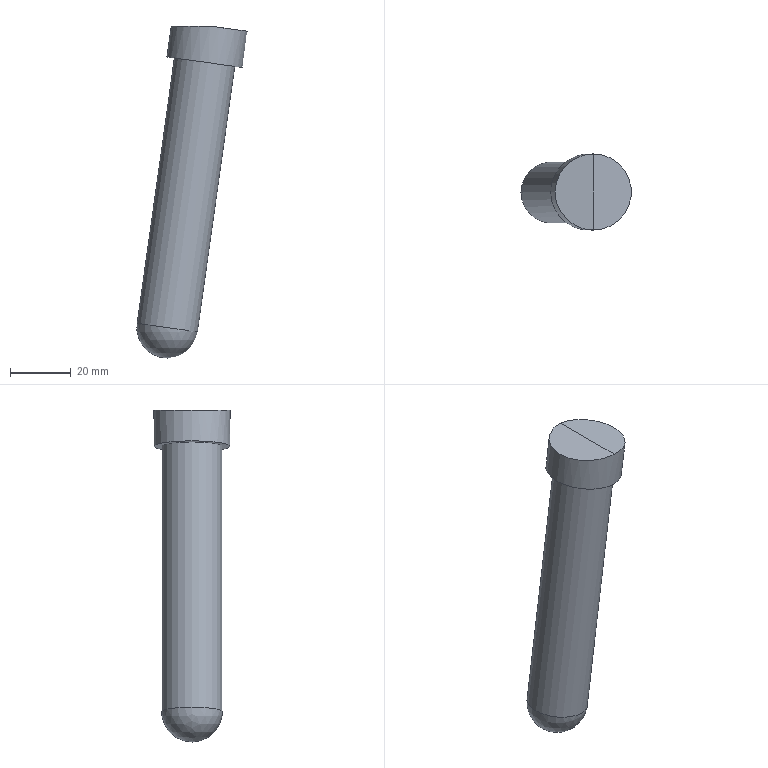Part | STEP file | P011002S003-011 | 1 solid | 6 faces | box 36.296 x 25 x 109.027 mm | volume 35448 mm3 | plane 3 | cylinder 2 | sphere 1 | commonest cylinder face diameters 20 x1 25 x1
STEP:
#1=CARTESIAN_POINT('',(0.,0.,0.));
#2=DIRECTION('',(0.,0.,1.));
#3=DIRECTION('',(1.,0.,0.));
#4=AXIS2_PLACEMENT_3D('',#1,#2,#3);
#5=CARTESIAN_POINT('',(-193.,-46.5,75.));
#6=VERTEX_POINT('',#5);
#7=CARTESIAN_POINT('',(-193.,-71.5,75.));
#8=VERTEX_POINT('',#7);
#9=CARTESIAN_POINT('',(-193.,-59.,75.));
#10=DIRECTION('',(0.,-1.,0.));
#11=VECTOR('',#10,1.);
#12=LINE('',#9,#11);
#13=CARTESIAN_POINT('',(-193.,-59.,75.));
#14=DIRECTION('',(-0.1392,0.,-0.9903));
#15=DIRECTION('',(0.9903,0.,-0.1392));
#16=AXIS2_PLACEMENT_3D('',#13,#14,#15);
#17=PLANE('',#16);
#18=CARTESIAN_POINT('',(0.,0.));
#19=DIRECTION('',(0.,1.));
#20=VECTOR('',#19,1.);
#21=LINE('',#18,#20);
#22=(GEOMETRIC_REPRESENTATION_CONTEXT(2)PARAMETRIC_REPRESENTATION_CONTEXT()REPRESENTATION_CONTEXT('',''));
#23=DEFINITIONAL_REPRESENTATION('',(#21),#22);
#24=PCURVE('',#17,#23);
#25=CARTESIAN_POINT('',(-250.,-9.,75.));
#26=DIRECTION('',(0.,0.,1.));
#27=DIRECTION('',(-1.,0.,0.));
#28=AXIS2_PLACEMENT_3D('',#25,#26,#27);
#29=PLANE('',#28);
#30=CARTESIAN_POINT('',(-57.,50.));
#31=DIRECTION('',(0.,1.));
#32=VECTOR('',#31,1.);
#33=LINE('',#30,#32);
#34=(GEOMETRIC_REPRESENTATION_CONTEXT(2)PARAMETRIC_REPRESENTATION_CONTEXT()REPRESENTATION_CONTEXT('',''));
#35=DEFINITIONAL_REPRESENTATION('',(#33),#34);
#36=PCURVE('',#29,#35);
#37=SURFACE_CURVE('',#12,(#24,#36),.PCURVE_S1.);
#38=EDGE_CURVE('',#6,#8,#37,.T.);
#39=ORIENTED_EDGE('',*,*,#38,.T.);
#40=CARTESIAN_POINT('',(-193.,-59.,75.));
#41=DIRECTION('',(0.1392,0.,0.9903));
#42=DIRECTION('',(0.9903,0.,-0.1392));
#43=AXIS2_PLACEMENT_3D('',#40,#41,#42);
#44=CIRCLE('',#43,12.5);
#45=CARTESIAN_POINT('',(12.5,0.));
#46=CARTESIAN_POINT('',(12.5,-21.651));
#47=CARTESIAN_POINT('',(-6.25,-10.825));
#48=CARTESIAN_POINT('',(-25.,0.));
#49=CARTESIAN_POINT('',(-6.25,10.825));
#50=CARTESIAN_POINT('',(12.5,21.651));
#51=CARTESIAN_POINT('',(12.5,0.));
#52=(BOUNDED_CURVE()B_SPLINE_CURVE(2,(#45,#46,#47,#48,#49,#50,#51),.UNSPECIFIED.,.T.,.F.)B_SPLINE_CURVE_WITH_KNOTS((1,2,2,2,2,1),(-2.094,0.,2.094,4.189,6.283,8.378),.UNSPECIFIED.)CURVE()GEOMETRIC_REPRESENTATION_ITEM()RATIONAL_B_SPLINE_CURVE((1.,0.5,1.,0.5,1.,0.5,1.))REPRESENTATION_ITEM(''));
#53=(GEOMETRIC_REPRESENTATION_CONTEXT(2)PARAMETRIC_REPRESENTATION_CONTEXT()REPRESENTATION_CONTEXT('',''));
#54=DEFINITIONAL_REPRESENTATION('',(#52),#53);
#55=PCURVE('',#17,#54);
#56=CARTESIAN_POINT('',(-222.706,-59.,-136.373));
#57=DIRECTION('',(0.1392,0.,0.9903));
#58=DIRECTION('',(-0.9903,0.,0.1392));
#59=AXIS2_PLACEMENT_3D('',#56,#57,#58);
#60=CYLINDRICAL_SURFACE('',#59,12.5);
#61=CARTESIAN_POINT('',(-3.142,213.45));
#62=DIRECTION('',(1.,0.));
#63=VECTOR('',#62,1.);
#64=LINE('',#61,#63);
#65=(GEOMETRIC_REPRESENTATION_CONTEXT(2)PARAMETRIC_REPRESENTATION_CONTEXT()REPRESENTATION_CONTEXT('',''));
#66=DEFINITIONAL_REPRESENTATION('',(#64),#65);
#67=PCURVE('',#60,#66);
#68=SURFACE_CURVE('',#44,(#55,#67),.PCURVE_S1.);
#69=EDGE_CURVE('',#8,#6,#68,.T.);
#70=ORIENTED_EDGE('',*,*,#69,.T.);
#71=EDGE_LOOP('',(#39,#70));
#72=FACE_BOUND('',#71,.T.);
#73=ADVANCED_FACE('',(#72),#17,.F.);
#74=CARTESIAN_POINT('',(-207.048,-59.,64.856));
#75=VERTEX_POINT('',#74);
#76=CARTESIAN_POINT('',(-194.67,-59.,63.117));
#77=DIRECTION('',(-0.1392,0.,-0.9903));
#78=DIRECTION('',(-0.9903,0.,0.1392));
#79=AXIS2_PLACEMENT_3D('',#76,#77,#78);
#80=CIRCLE('',#79,12.5);
#81=CARTESIAN_POINT('',(6.283,201.45));
#82=DIRECTION('',(-1.,0.));
#83=VECTOR('',#82,1.);
#84=LINE('',#81,#83);
#85=(GEOMETRIC_REPRESENTATION_CONTEXT(2)PARAMETRIC_REPRESENTATION_CONTEXT()REPRESENTATION_CONTEXT('',''));
#86=DEFINITIONAL_REPRESENTATION('',(#84),#85);
#87=PCURVE('',#60,#86);
#88=CARTESIAN_POINT('',(-194.67,-109.,63.117));
#89=DIRECTION('',(0.1392,0.,0.9903));
#90=DIRECTION('',(-0.9903,0.,0.1392));
#91=AXIS2_PLACEMENT_3D('',#88,#89,#90);
#92=PLANE('',#91);
#93=CARTESIAN_POINT('',(12.5,-50.));
#94=CARTESIAN_POINT('',(12.5,-71.651));
#95=CARTESIAN_POINT('',(-6.25,-60.825));
#96=CARTESIAN_POINT('',(-25.,-50.));
#97=CARTESIAN_POINT('',(-6.25,-39.175));
#98=CARTESIAN_POINT('',(12.5,-28.349));
#99=CARTESIAN_POINT('',(12.5,-50.));
#100=(BOUNDED_CURVE()B_SPLINE_CURVE(2,(#93,#94,#95,#96,#97,#98,#99),.UNSPECIFIED.,.T.,.F.)B_SPLINE_CURVE_WITH_KNOTS((1,2,2,2,2,1),(-2.094,0.,2.094,4.189,6.283,8.378),.UNSPECIFIED.)CURVE()GEOMETRIC_REPRESENTATION_ITEM()RATIONAL_B_SPLINE_CURVE((1.,0.5,1.,0.5,1.,0.5,1.))REPRESENTATION_ITEM(''));
#101=(GEOMETRIC_REPRESENTATION_CONTEXT(2)PARAMETRIC_REPRESENTATION_CONTEXT()REPRESENTATION_CONTEXT('',''));
#102=DEFINITIONAL_REPRESENTATION('',(#100),#101);
#103=PCURVE('',#92,#102);
#104=SURFACE_CURVE('',#80,(#87,#103),.PCURVE_S1.);
#105=EDGE_CURVE('',#75,#75,#104,.T.);
#106=ORIENTED_EDGE('',*,*,#105,.F.);
#107=CARTESIAN_POINT('',(-205.623,-59.,75.));
#108=VERTEX_POINT('',#107);
#109=CARTESIAN_POINT('',(-207.048,-59.,64.856));
#110=CARTESIAN_POINT('',(-205.623,-59.,75.));
#111=B_SPLINE_CURVE_WITH_KNOTS('',1,(#109,#110),.UNSPECIFIED.,.F.,.F.,(2,2),(201.45,211.693),.PIECEWISE_BEZIER_KNOTS.);
#112=CARTESIAN_POINT('',(6.283,0.));
#113=DIRECTION('',(0.,1.));
#114=VECTOR('',#113,1.);
#115=LINE('',#112,#114);
#116=(GEOMETRIC_REPRESENTATION_CONTEXT(2)PARAMETRIC_REPRESENTATION_CONTEXT()REPRESENTATION_CONTEXT('',''));
#117=DEFINITIONAL_REPRESENTATION('',(#115),#116);
#118=PCURVE('',#60,#117);
#119=CARTESIAN_POINT('',(0.,0.));
#120=DIRECTION('',(0.,1.));
#121=VECTOR('',#120,1.);
#122=LINE('',#119,#121);
#123=(GEOMETRIC_REPRESENTATION_CONTEXT(2)PARAMETRIC_REPRESENTATION_CONTEXT()REPRESENTATION_CONTEXT('',''));
#124=DEFINITIONAL_REPRESENTATION('',(#122),#123);
#125=PCURVE('',#60,#124);
#126=SEAM_CURVE('',#111,(#118,#125),.PCURVE_S1.);
#127=EDGE_CURVE('',#75,#108,#126,.T.);
#128=ORIENTED_EDGE('',*,*,#127,.T.);
#129=CARTESIAN_POINT('',(-193.,-59.,75.));
#130=DIRECTION('',(0.,0.,-1.));
#131=DIRECTION('',(1.,0.,0.));
#132=AXIS2_PLACEMENT_3D('',#129,#130,#131);
#133=ELLIPSE('',#132,12.623,12.5);
#134=CARTESIAN_POINT('',(7.854,213.45));
#135=CARTESIAN_POINT('',(7.806,213.366));
#136=CARTESIAN_POINT('',(7.711,213.199));
#137=CARTESIAN_POINT('',(7.568,212.953));
#138=CARTESIAN_POINT('',(7.426,212.718));
#139=CARTESIAN_POINT('',(7.283,212.497));
#140=CARTESIAN_POINT('',(7.14,212.296));
#141=CARTESIAN_POINT('',(6.997,212.118));
#142=CARTESIAN_POINT('',(6.854,211.967));
#143=CARTESIAN_POINT('',(6.712,211.846));
#144=CARTESIAN_POINT('',(6.569,211.759));
#145=CARTESIAN_POINT('',(6.426,211.705));
#146=CARTESIAN_POINT('',(6.283,211.687));
#147=CARTESIAN_POINT('',(6.14,211.705));
#148=CARTESIAN_POINT('',(5.998,211.759));
#149=CARTESIAN_POINT('',(5.855,211.846));
#150=CARTESIAN_POINT('',(5.712,211.967));
#151=CARTESIAN_POINT('',(5.569,212.118));
#152=CARTESIAN_POINT('',(5.426,212.296));
#153=CARTESIAN_POINT('',(5.284,212.497));
#154=CARTESIAN_POINT('',(5.141,212.718));
#155=CARTESIAN_POINT('',(4.998,212.953));
#156=CARTESIAN_POINT('',(4.855,213.199));
#157=CARTESIAN_POINT('',(4.76,213.366));
#158=CARTESIAN_POINT('',(4.712,213.45));
#159=B_SPLINE_CURVE_WITH_KNOTS('',3,(#134,#135,#136,#137,#138,#139,#140,#141,#142,#143,#144,#145,#146,#147,#148,#149,#150,#151,#152,#153,#154,#155,#156,#157,#158),.UNSPECIFIED.,.F.,.F.,(4,1,1,1,1,1,1,1,1,1,1,1,1,1,1,1,1,1,1,1,1,1,4),(1.571,1.714,1.856,1.999,2.142,2.285,2.428,2.57,2.713,2.856,2.999,3.142,3.284,3.427,3.57,3.713,3.856,3.998,4.141,4.284,4.427,4.57,4.712),.QUASI_UNIFORM_KNOTS.);
#160=(GEOMETRIC_REPRESENTATION_CONTEXT(2)PARAMETRIC_REPRESENTATION_CONTEXT()REPRESENTATION_CONTEXT('',''));
#161=DEFINITIONAL_REPRESENTATION('',(#159),#160);
#162=PCURVE('',#60,#161);
#163=CARTESIAN_POINT('',(-69.623,50.));
#164=CARTESIAN_POINT('',(-69.623,71.651));
#165=CARTESIAN_POINT('',(-50.689,60.825));
#166=CARTESIAN_POINT('',(-31.754,50.));
#167=CARTESIAN_POINT('',(-50.689,39.175));
#168=CARTESIAN_POINT('',(-69.623,28.349));
#169=CARTESIAN_POINT('',(-69.623,50.));
#170=(BOUNDED_CURVE()B_SPLINE_CURVE(2,(#163,#164,#165,#166,#167,#168,#169),.UNSPECIFIED.,.T.,.F.)B_SPLINE_CURVE_WITH_KNOTS((1,2,2,2,2,1),(-2.094,0.,2.094,4.189,6.283,8.378),.UNSPECIFIED.)CURVE()GEOMETRIC_REPRESENTATION_ITEM()RATIONAL_B_SPLINE_CURVE((1.,0.5,1.,0.5,1.,0.5,1.))REPRESENTATION_ITEM(''));
#171=(GEOMETRIC_REPRESENTATION_CONTEXT(2)PARAMETRIC_REPRESENTATION_CONTEXT()REPRESENTATION_CONTEXT('',''));
#172=DEFINITIONAL_REPRESENTATION('',(#170),#171);
#173=PCURVE('',#29,#172);
#174=SURFACE_CURVE('',#133,(#162,#173),.PCURVE_S1.);
#175=EDGE_CURVE('',#108,#6,#174,.T.);
#176=ORIENTED_EDGE('',*,*,#175,.T.);
#177=ORIENTED_EDGE('',*,*,#69,.F.);
#178=CARTESIAN_POINT('',(-193.,-59.,75.));
#179=DIRECTION('',(0.,0.,-1.));
#180=DIRECTION('',(1.,0.,0.));
#181=AXIS2_PLACEMENT_3D('',#178,#179,#180);
#182=ELLIPSE('',#181,12.623,12.5);
#183=CARTESIAN_POINT('',(1.571,213.45));
#184=CARTESIAN_POINT('',(1.523,213.366));
#185=CARTESIAN_POINT('',(1.428,213.199));
#186=CARTESIAN_POINT('',(1.285,212.953));
#187=CARTESIAN_POINT('',(1.142,212.718));
#188=CARTESIAN_POINT('',(0.9996,212.497));
#189=CARTESIAN_POINT('',(0.8568,212.296));
#190=CARTESIAN_POINT('',(0.714,212.118));
#191=CARTESIAN_POINT('',(0.5712,211.967));
#192=CARTESIAN_POINT('',(0.4284,211.846));
#193=CARTESIAN_POINT('',(0.2856,211.759));
#194=CARTESIAN_POINT('',(0.1428,211.705));
#195=CARTESIAN_POINT('',(0.,211.687));
#196=CARTESIAN_POINT('',(-0.1428,211.705));
#197=CARTESIAN_POINT('',(-0.2856,211.759));
#198=CARTESIAN_POINT('',(-0.4284,211.846));
#199=CARTESIAN_POINT('',(-0.5712,211.967));
#200=CARTESIAN_POINT('',(-0.714,212.118));
#201=CARTESIAN_POINT('',(-0.8568,212.296));
#202=CARTESIAN_POINT('',(-0.9996,212.497));
#203=CARTESIAN_POINT('',(-1.142,212.718));
#204=CARTESIAN_POINT('',(-1.285,212.953));
#205=CARTESIAN_POINT('',(-1.428,213.199));
#206=CARTESIAN_POINT('',(-1.523,213.366));
#207=CARTESIAN_POINT('',(-1.571,213.45));
#208=B_SPLINE_CURVE_WITH_KNOTS('',3,(#183,#184,#185,#186,#187,#188,#189,#190,#191,#192,#193,#194,#195,#196,#197,#198,#199,#200,#201,#202,#203,#204,#205,#206,#207),.UNSPECIFIED.,.F.,.F.,(4,1,1,1,1,1,1,1,1,1,1,1,1,1,1,1,1,1,1,1,1,1,4),(1.571,1.714,1.856,1.999,2.142,2.285,2.428,2.57,2.713,2.856,2.999,3.142,3.284,3.427,3.57,3.713,3.856,3.998,4.141,4.284,4.427,4.57,4.712),.QUASI_UNIFORM_KNOTS.);
#209=(GEOMETRIC_REPRESENTATION_CONTEXT(2)PARAMETRIC_REPRESENTATION_CONTEXT()REPRESENTATION_CONTEXT('',''));
#210=DEFINITIONAL_REPRESENTATION('',(#208),#209);
#211=PCURVE('',#60,#210);
#212=CARTESIAN_POINT('',(-69.623,50.));
#213=CARTESIAN_POINT('',(-69.623,71.651));
#214=CARTESIAN_POINT('',(-50.689,60.825));
#215=CARTESIAN_POINT('',(-31.754,50.));
#216=CARTESIAN_POINT('',(-50.689,39.175));
#217=CARTESIAN_POINT('',(-69.623,28.349));
#218=CARTESIAN_POINT('',(-69.623,50.));
#219=(BOUNDED_CURVE()B_SPLINE_CURVE(2,(#212,#213,#214,#215,#216,#217,#218),.UNSPECIFIED.,.T.,.F.)B_SPLINE_CURVE_WITH_KNOTS((1,2,2,2,2,1),(-2.094,0.,2.094,4.189,6.283,8.378),.UNSPECIFIED.)CURVE()GEOMETRIC_REPRESENTATION_ITEM()RATIONAL_B_SPLINE_CURVE((1.,0.5,1.,0.5,1.,0.5,1.))REPRESENTATION_ITEM(''));
#220=(GEOMETRIC_REPRESENTATION_CONTEXT(2)PARAMETRIC_REPRESENTATION_CONTEXT()REPRESENTATION_CONTEXT('',''));
#221=DEFINITIONAL_REPRESENTATION('',(#219),#220);
#222=PCURVE('',#29,#221);
#223=SURFACE_CURVE('',#182,(#211,#222),.PCURVE_S1.);
#224=EDGE_CURVE('',#8,#108,#223,.T.);
#225=ORIENTED_EDGE('',*,*,#224,.T.);
#226=ORIENTED_EDGE('',*,*,#127,.F.);
#227=EDGE_LOOP('',(#106,#128,#176,#177,#225,#226));
#228=FACE_BOUND('',#227,.T.);
#229=ADVANCED_FACE('',(#228),#60,.T.);
#230=CARTESIAN_POINT('',(-216.82,-59.,-22.635));
#231=VERTEX_POINT('',#230);
#232=CARTESIAN_POINT('',(-206.917,-59.,-24.027));
#233=DIRECTION('',(-0.1392,0.,-0.9903));
#234=DIRECTION('',(-0.9903,0.,0.1392));
#235=AXIS2_PLACEMENT_3D('',#232,#233,#234);
#236=CIRCLE('',#235,10.);
#237=CARTESIAN_POINT('',(-222.706,-59.,-136.373));
#238=DIRECTION('',(0.1392,0.,0.9903));
#239=DIRECTION('',(-0.9903,0.,0.1392));
#240=AXIS2_PLACEMENT_3D('',#237,#238,#239);
#241=CYLINDRICAL_SURFACE('',#240,10.);
#242=CARTESIAN_POINT('',(6.283,113.45));
#243=DIRECTION('',(-1.,0.));
#244=VECTOR('',#243,1.);
#245=LINE('',#242,#244);
#246=(GEOMETRIC_REPRESENTATION_CONTEXT(2)PARAMETRIC_REPRESENTATION_CONTEXT()REPRESENTATION_CONTEXT('',''));
#247=DEFINITIONAL_REPRESENTATION('',(#245),#246);
#248=PCURVE('',#241,#247);
#249=CARTESIAN_POINT('',(-206.917,-59.,-24.027));
#250=DIRECTION('',(0.,0.,1.));
#251=DIRECTION('',(-1.,0.,0.));
#252=AXIS2_PLACEMENT_3D('',#249,#250,#251);
#253=SPHERICAL_SURFACE('',#252,10.);
#254=CARTESIAN_POINT('',(6.283,0.1396));
#255=CARTESIAN_POINT('',(6.187,0.1397));
#256=CARTESIAN_POINT('',(5.995,0.1357));
#257=CARTESIAN_POINT('',(5.707,0.119));
#258=CARTESIAN_POINT('',(5.421,0.0925));
#259=CARTESIAN_POINT('',(5.137,0.05863));
#260=CARTESIAN_POINT('',(4.854,0.02007));
#261=CARTESIAN_POINT('',(4.571,-0.02007));
#262=CARTESIAN_POINT('',(4.288,-0.05863));
#263=CARTESIAN_POINT('',(4.003,-0.0925));
#264=CARTESIAN_POINT('',(3.717,-0.119));
#265=CARTESIAN_POINT('',(3.43,-0.1358));
#266=CARTESIAN_POINT('',(3.142,-0.1416));
#267=CARTESIAN_POINT('',(2.853,-0.1358));
#268=CARTESIAN_POINT('',(2.566,-0.119));
#269=CARTESIAN_POINT('',(2.28,-0.0925));
#270=CARTESIAN_POINT('',(1.995,-0.05863));
#271=CARTESIAN_POINT('',(1.712,-0.02007));
#272=CARTESIAN_POINT('',(1.429,0.02007));
#273=CARTESIAN_POINT('',(1.146,0.05863));
#274=CARTESIAN_POINT('',(0.8619,0.0925));
#275=CARTESIAN_POINT('',(0.5759,0.119));
#276=CARTESIAN_POINT('',(0.2884,0.1357));
#277=CARTESIAN_POINT('',(0.09616,0.1397));
#278=CARTESIAN_POINT('',(0.,0.1396));
#279=B_SPLINE_CURVE_WITH_KNOTS('',3,(#254,#255,#256,#257,#258,#259,#260,#261,#262,#263,#264,#265,#266,#267,#268,#269,#270,#271,#272,#273,#274,#275,#276,#277,#278),.UNSPECIFIED.,.F.,.F.,(4,1,1,1,1,1,1,1,1,1,1,1,1,1,1,1,1,1,1,1,1,1,4),(0.,0.2856,0.5712,0.8568,1.142,1.428,1.714,1.999,2.285,2.57,2.856,3.142,3.427,3.713,3.998,4.284,4.57,4.855,5.141,5.426,5.712,5.998,6.283),.QUASI_UNIFORM_KNOTS.);
#280=(GEOMETRIC_REPRESENTATION_CONTEXT(2)PARAMETRIC_REPRESENTATION_CONTEXT()REPRESENTATION_CONTEXT('',''));
#281=DEFINITIONAL_REPRESENTATION('',(#279),#280);
#282=PCURVE('',#253,#281);
#283=SURFACE_CURVE('',#236,(#248,#282),.PCURVE_S1.);
#284=EDGE_CURVE('',#231,#231,#283,.T.);
#285=ORIENTED_EDGE('',*,*,#284,.F.);
#286=CARTESIAN_POINT('',(-204.573,-59.,64.509));
#287=VERTEX_POINT('',#286);
#288=CARTESIAN_POINT('',(-216.82,-59.,-22.635));
#289=CARTESIAN_POINT('',(-204.573,-59.,64.509));
#290=B_SPLINE_CURVE_WITH_KNOTS('',1,(#288,#289),.UNSPECIFIED.,.F.,.F.,(2,2),(113.45,201.45),.PIECEWISE_BEZIER_KNOTS.);
#291=CARTESIAN_POINT('',(6.283,0.));
#292=DIRECTION('',(0.,1.));
#293=VECTOR('',#292,1.);
#294=LINE('',#291,#293);
#295=(GEOMETRIC_REPRESENTATION_CONTEXT(2)PARAMETRIC_REPRESENTATION_CONTEXT()REPRESENTATION_CONTEXT('',''));
#296=DEFINITIONAL_REPRESENTATION('',(#294),#295);
#297=PCURVE('',#241,#296);
#298=CARTESIAN_POINT('',(0.,0.));
#299=DIRECTION('',(0.,1.));
#300=VECTOR('',#299,1.);
#301=LINE('',#298,#300);
#302=(GEOMETRIC_REPRESENTATION_CONTEXT(2)PARAMETRIC_REPRESENTATION_CONTEXT()REPRESENTATION_CONTEXT('',''));
#303=DEFINITIONAL_REPRESENTATION('',(#301),#302);
#304=PCURVE('',#241,#303);
#305=SEAM_CURVE('',#290,(#297,#304),.PCURVE_S1.);
#306=EDGE_CURVE('',#231,#287,#305,.T.);
#307=ORIENTED_EDGE('',*,*,#306,.T.);
#308=CARTESIAN_POINT('',(-194.67,-59.,63.117));
#309=DIRECTION('',(-0.1392,0.,-0.9903));
#310=DIRECTION('',(-0.9903,0.,0.1392));
#311=AXIS2_PLACEMENT_3D('',#308,#309,#310);
#312=CIRCLE('',#311,10.);
#313=CARTESIAN_POINT('',(6.283,201.45));
#314=DIRECTION('',(-1.,0.));
#315=VECTOR('',#314,1.);
#316=LINE('',#313,#315);
#317=(GEOMETRIC_REPRESENTATION_CONTEXT(2)PARAMETRIC_REPRESENTATION_CONTEXT()REPRESENTATION_CONTEXT('',''));
#318=DEFINITIONAL_REPRESENTATION('',(#316),#317);
#319=PCURVE('',#241,#318);
#320=CARTESIAN_POINT('',(10.,-50.));
#321=CARTESIAN_POINT('',(10.,-67.321));
#322=CARTESIAN_POINT('',(-5.,-58.66));
#323=CARTESIAN_POINT('',(-20.,-50.));
#324=CARTESIAN_POINT('',(-5.,-41.34));
#325=CARTESIAN_POINT('',(10.,-32.679));
#326=CARTESIAN_POINT('',(10.,-50.));
#327=(BOUNDED_CURVE()B_SPLINE_CURVE(2,(#320,#321,#322,#323,#324,#325,#326),.UNSPECIFIED.,.T.,.F.)B_SPLINE_CURVE_WITH_KNOTS((1,2,2,2,2,1),(-2.094,0.,2.094,4.189,6.283,8.378),.UNSPECIFIED.)CURVE()GEOMETRIC_REPRESENTATION_ITEM()RATIONAL_B_SPLINE_CURVE((1.,0.5,1.,0.5,1.,0.5,1.))REPRESENTATION_ITEM(''));
#328=(GEOMETRIC_REPRESENTATION_CONTEXT(2)PARAMETRIC_REPRESENTATION_CONTEXT()REPRESENTATION_CONTEXT('',''));
#329=DEFINITIONAL_REPRESENTATION('',(#327),#328);
#330=PCURVE('',#92,#329);
#331=SURFACE_CURVE('',#312,(#319,#330),.PCURVE_S1.);
#332=EDGE_CURVE('',#287,#287,#331,.T.);
#333=ORIENTED_EDGE('',*,*,#332,.T.);
#334=ORIENTED_EDGE('',*,*,#306,.F.);
#335=EDGE_LOOP('',(#285,#307,#333,#334));
#336=FACE_BOUND('',#335,.T.);
#337=ADVANCED_FACE('',(#336),#241,.T.);
#338=ORIENTED_EDGE('',*,*,#105,.T.);
#339=EDGE_LOOP('',(#338));
#340=FACE_BOUND('',#339,.T.);
#341=ORIENTED_EDGE('',*,*,#332,.F.);
#342=EDGE_LOOP('',(#341));
#343=FACE_BOUND('',#342,.T.);
#344=ADVANCED_FACE('',(#340,#343),#92,.F.);
#345=ORIENTED_EDGE('',*,*,#284,.T.);
#346=CARTESIAN_POINT('',(-206.917,-59.,-34.027));
#347=VERTEX_POINT('',#346);
#348=CARTESIAN_POINT('',(-206.917,-59.,-34.027));
#349=CARTESIAN_POINT('',(-209.361,-59.,-34.027));
#350=CARTESIAN_POINT('',(-211.804,-59.,-33.33));
#351=CARTESIAN_POINT('',(-214.01,-59.,-31.937));
#352=CARTESIAN_POINT('',(-215.738,-59.,-29.949));
#353=CARTESIAN_POINT('',(-216.81,-59.,-27.571));
#354=CARTESIAN_POINT('',(-217.16,-59.,-25.055));
#355=CARTESIAN_POINT('',(-216.82,-59.,-22.635));
#356=B_SPLINE_CURVE_WITH_KNOTS('',7,(#348,#349,#350,#351,#352,#353,#354,#355),.UNSPECIFIED.,.F.,.F.,(8,8),(-1.571,0.1396),.PIECEWISE_BEZIER_KNOTS.);
#357=CARTESIAN_POINT('',(0.,0.));
#358=DIRECTION('',(0.,1.));
#359=VECTOR('',#358,1.);
#360=LINE('',#357,#359);
#361=(GEOMETRIC_REPRESENTATION_CONTEXT(2)PARAMETRIC_REPRESENTATION_CONTEXT()REPRESENTATION_CONTEXT('',''));
#362=DEFINITIONAL_REPRESENTATION('',(#360),#361);
#363=PCURVE('',#253,#362);
#364=CARTESIAN_POINT('',(6.283,0.));
#365=DIRECTION('',(0.,1.));
#366=VECTOR('',#365,1.);
#367=LINE('',#364,#366);
#368=(GEOMETRIC_REPRESENTATION_CONTEXT(2)PARAMETRIC_REPRESENTATION_CONTEXT()REPRESENTATION_CONTEXT('',''));
#369=DEFINITIONAL_REPRESENTATION('',(#367),#368);
#370=PCURVE('',#253,#369);
#371=SEAM_CURVE('',#356,(#363,#370),.PCURVE_S1.);
#372=EDGE_CURVE('',#347,#231,#371,.T.);
#373=ORIENTED_EDGE('',*,*,#372,.F.);
#374=ORIENTED_EDGE('',*,*,#372,.T.);
#375=EDGE_LOOP('',(#345,#373,#374));
#376=FACE_BOUND('',#375,.T.);
#377=ADVANCED_FACE('',(#376),#253,.T.);
#378=ORIENTED_EDGE('',*,*,#224,.F.);
#379=ORIENTED_EDGE('',*,*,#38,.F.);
#380=ORIENTED_EDGE('',*,*,#175,.F.);
#381=EDGE_LOOP('',(#378,#379,#380));
#382=FACE_BOUND('',#381,.T.);
#383=ADVANCED_FACE('',(#382),#29,.T.);
#384=CLOSED_SHELL('',(#73,#229,#337,#344,#377,#383));
#385=MANIFOLD_SOLID_BREP('',#384);
#386=(LENGTH_UNIT()NAMED_UNIT(*)SI_UNIT(.MILLI.,.METRE.));
#387=UNCERTAINTY_MEASURE_WITH_UNIT(LENGTH_MEASURE(0.000005),#386,'','');
#388=(NAMED_UNIT(*)PLANE_ANGLE_UNIT()SI_UNIT($,.RADIAN.));
#389=(NAMED_UNIT(*)SI_UNIT($,.STERADIAN.)SOLID_ANGLE_UNIT());
#390=(GEOMETRIC_REPRESENTATION_CONTEXT(3)GLOBAL_UNCERTAINTY_ASSIGNED_CONTEXT((#387))GLOBAL_UNIT_ASSIGNED_CONTEXT((#386,#388,#389))REPRESENTATION_CONTEXT('',''));
#391=ADVANCED_BREP_SHAPE_REPRESENTATION('',(#4,#385),#390);